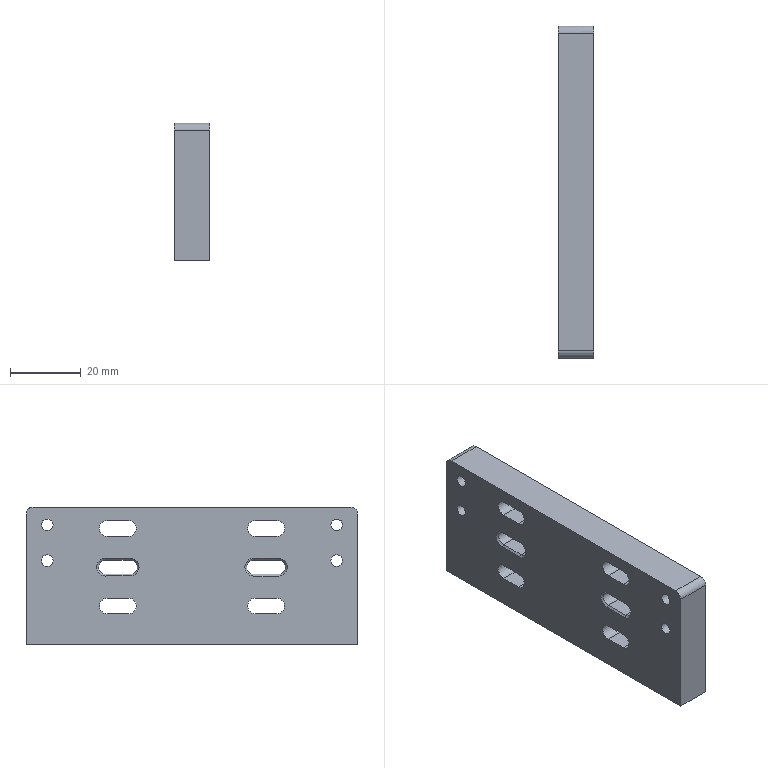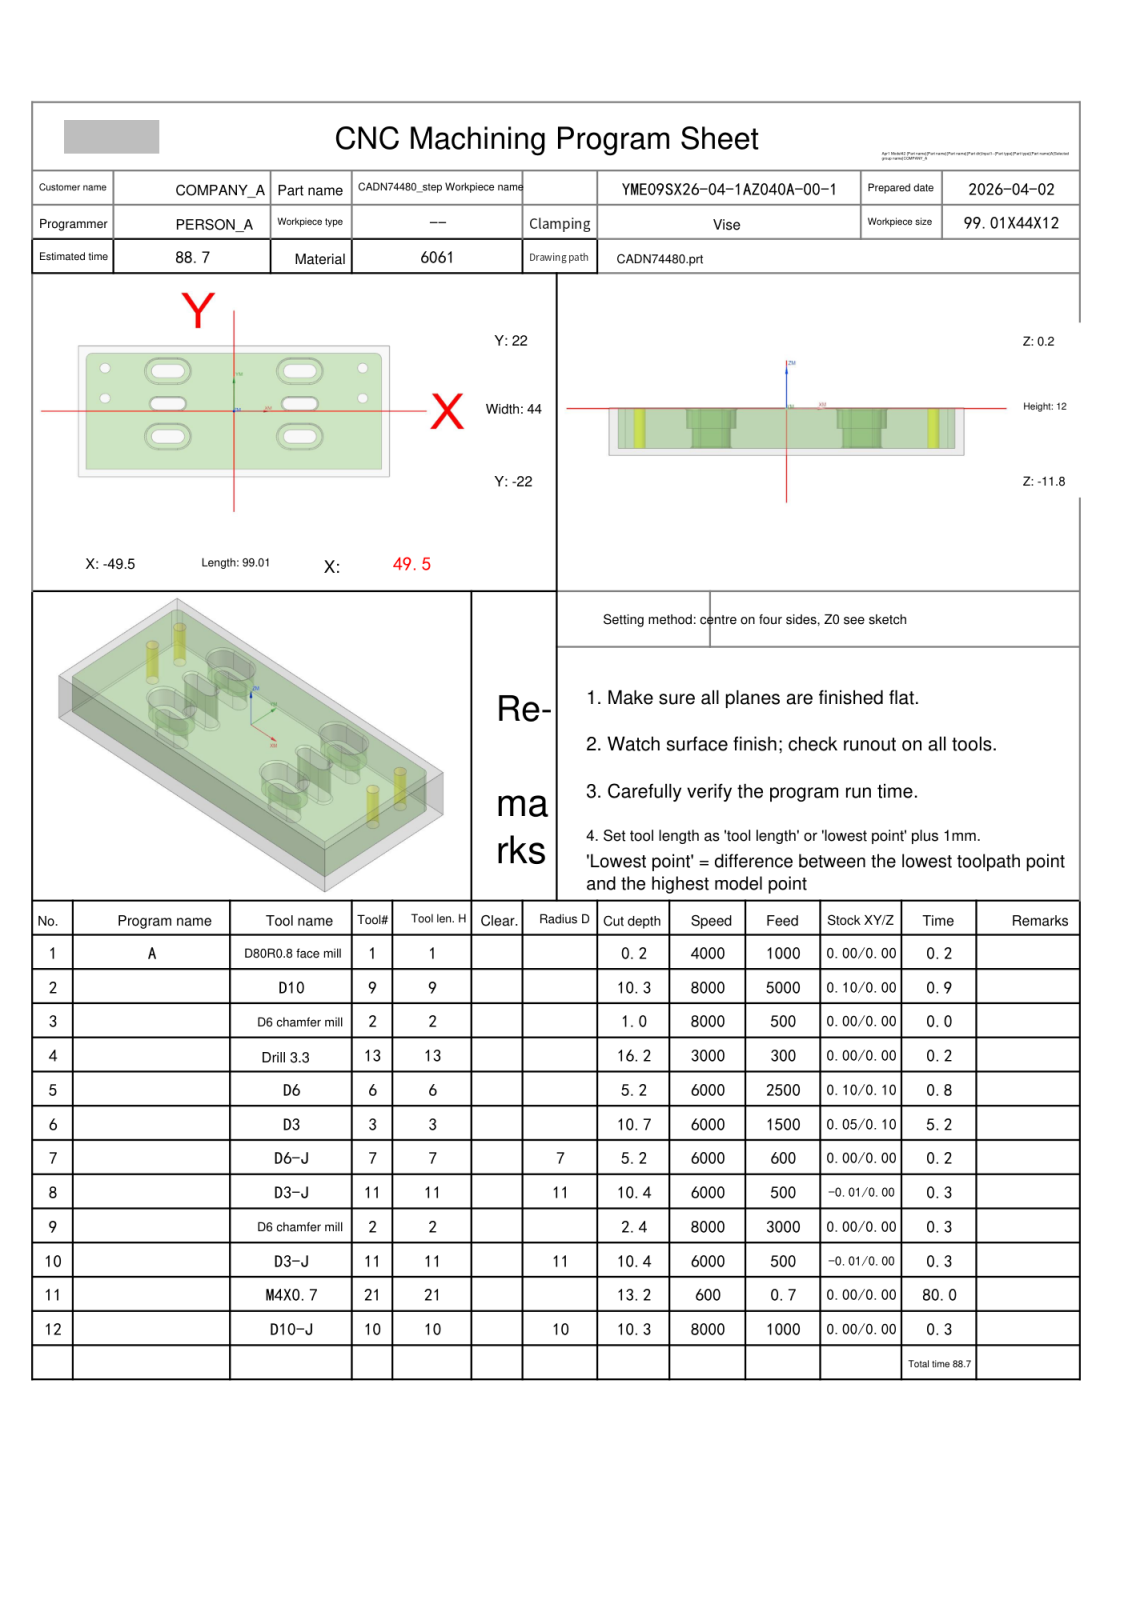NC program | NX | posted by the shop | part box 10.067 x 94 x 39 mm
Lines 3804 to 4590 of 4590:
N7 T07 M06
(D6-J  D=6. R=0. H=07 ce=0.00 di=0.00)
G00 G90 G54 X-21.196 Y-9.25 M03 S6000
G43 H07 Z20.
M08
Z-4.5
G01 Z-5. F600.
G41 D07
Y-9.3
G03 X-20.996 Y-9.5 I.2 J0.0
G01 X-17.996
G03 X-16.996 Y-8.5 I0.0 J1.
X-17.996 Y-7.5 I-1. J0.0
G01 X-23.996
G03 X-24.996 Y-8.5 I0.0 J-1.
X-23.996 Y-9.5 I1. J0.0
G01 X-20.996
X-20.496
G03 X-20.296 Y-9.3 I0.0 J.2
G01 G40 Y-9.25
Z-4.5
G00 Z20.
X-20.796 Y14.25
Z-4.5
G01 Z-5.
G41 D07
Y14.3
G03 X-20.996 Y14.5 I-.2 J0.0
G01 X-23.996
G03 X-24.996 Y13.5 I0.0 J-1.
X-23.996 Y12.5 I1. J0.0
G01 X-17.996
G03 X-16.996 Y13.5 I0.0 J1.
X-17.996 Y14.5 I-1. J0.0
G01 X-20.996
X-21.496
G03 X-21.696 Y14.3 I0.0 J-.2
G01 G40 Y14.25
Z-4.5
G00 Z20.
X21.204
Z-4.5
G01 Z-5.
G41 D07
Y14.3
G03 X21.004 Y14.5 I-.2 J0.0
G01 X18.004
G03 X17.004 Y13.5 I0.0 J-1.
X18.004 Y12.5 I1. J0.0
G01 X24.004
G03 X25.004 Y13.5 I0.0 J1.
X24.004 Y14.5 I-1. J0.0
G01 X21.004
X20.504
G03 X20.304 Y14.3 I0.0 J-.2
G01 G40 Y14.25
Z-4.5
G00 Z20.
X20.804 Y-9.25
Z-4.5
G01 Z-5.
G41 D07
Y-9.3
G03 X21.004 Y-9.5 I.2 J0.0
G01 X24.004
G03 X25.004 Y-8.5 I0.0 J1.
X24.004 Y-7.5 I-1. J0.0
G01 X18.004
G03 X17.004 Y-8.5 I0.0 J-1.
X18.004 Y-9.5 I1. J0.0
G01 X21.004
X21.504
G03 X21.704 Y-9.3 I0.0 J.2
G01 G40 Y-9.25
Z-4.5
G00 Z20.
G91 G28 Z0.0
M05
M09
G91 G28 Z0.0
M01
N8 T11 M06
(D3-J  D=3. R=0. H=11 ce=-0.01 di=0.00)
G00 G90 G54 X-20.796 Y14.01 M03 S6000
G43 H11 Z20.
M08
Z-7.1
G01 Z-7.6 F500.
G41 D07
Y14.06
G03 X-20.996 Y14.26 I-.2 J0.0
G01 X-23.996
G03 X-24.756 Y13.5 I0.0 J-.76
X-23.996 Y12.74 I.76 J0.0
G01 X-17.996
G03 X-17.236 Y13.5 I0.0 J.76
X-17.996 Y14.26 I-.76 J0.0
G01 X-20.996
X-21.496
G03 X-21.696 Y14.06 I0.0 J-.2
G01 G40 Y14.01
Z-7.1
G00 Z-4.
X-20.796
Z-9.7
G01 Z-10.2
G41 D07
Y14.06
G03 X-20.996 Y14.26 I-.2 J0.0
G01 X-23.996
G03 X-24.756 Y13.5 I0.0 J-.76
X-23.996 Y12.74 I.76 J0.0
G01 X-17.996
G03 X-17.236 Y13.5 I0.0 J.76
X-17.996 Y14.26 I-.76 J0.0
G01 X-20.996
X-21.496
G03 X-21.696 Y14.06 I0.0 J-.2
G01 G40 Y14.01
Z-9.7
G00 Z20.
X-21.196 Y-9.01
Z-7.1
G01 Z-7.6
G41 D07
Y-9.06
G03 X-20.996 Y-9.26 I.2 J0.0
G01 X-17.996
G03 X-17.236 Y-8.5 I0.0 J.76
X-17.996 Y-7.74 I-.76 J0.0
G01 X-23.996
G03 X-24.756 Y-8.5 I0.0 J-.76
X-23.996 Y-9.26 I.76 J0.0
G01 X-20.996
X-20.496
G03 X-20.296 Y-9.06 I0.0 J.2
G01 G40 Y-9.01
Z-7.1
G00 Z-4.
X-21.196
Z-9.7
G01 Z-10.2
G41 D07
Y-9.06
G03 X-20.996 Y-9.26 I.2 J0.0
G01 X-17.996
G03 X-17.236 Y-8.5 I0.0 J.76
X-17.996 Y-7.74 I-.76 J0.0
G01 X-23.996
G03 X-24.756 Y-8.5 I0.0 J-.76
X-23.996 Y-9.26 I.76 J0.0
G01 X-20.996
X-20.496
G03 X-20.296 Y-9.06 I0.0 J.2
G01 G40 Y-9.01
Z-9.7
G00 Z20.
X20.804
Z-7.1
G01 Z-7.6
G41 D07
Y-9.06
G03 X21.004 Y-9.26 I.2 J0.0
G01 X24.004
G03 X24.764 Y-8.5 I0.0 J.76
X24.004 Y-7.74 I-.76 J0.0
G01 X18.004
G03 X17.244 Y-8.5 I0.0 J-.76
X18.004 Y-9.26 I.76 J0.0
G01 X21.004
X21.504
G03 X21.704 Y-9.06 I0.0 J.2
G01 G40 Y-9.01
Z-7.1
G00 Z-4.
X20.804
Z-9.7
G01 Z-10.2
G41 D07
Y-9.06
G03 X21.004 Y-9.26 I.2 J0.0
G01 X24.004
G03 X24.764 Y-8.5 I0.0 J.76
X24.004 Y-7.74 I-.76 J0.0
G01 X18.004
G03 X17.244 Y-8.5 I0.0 J-.76
X18.004 Y-9.26 I.76 J0.0
G01 X21.004
X21.504
G03 X21.704 Y-9.06 I0.0 J.2
G01 G40 Y-9.01
Z-9.7
G00 Z20.
X21.204 Y14.01
Z-7.1
G01 Z-7.6
G41 D07
Y14.06
G03 X21.004 Y14.26 I-.2 J0.0
G01 X18.004
G03 X17.244 Y13.5 I0.0 J-.76
X18.004 Y12.74 I.76 J0.0
G01 X24.004
G03 X24.764 Y13.5 I0.0 J.76
X24.004 Y14.26 I-.76 J0.0
G01 X21.004
X20.504
G03 X20.304 Y14.06 I0.0 J-.2
G01 G40 Y14.01
Z-7.1
G00 Z-4.
X21.204
Z-9.7
G01 Z-10.2
G41 D07
Y14.06
G03 X21.004 Y14.26 I-.2 J0.0
G01 X18.004
G03 X17.244 Y13.5 I0.0 J-.76
X18.004 Y12.74 I.76 J0.0
G01 X24.004
G03 X24.764 Y13.5 I0.0 J.76
X24.004 Y14.26 I-.76 J0.0
G01 X21.004
X20.504
G03 X20.304 Y14.06 I0.0 J-.2
G01 G40 Y14.01
Z-9.7
G00 Z20.
G91 G28 Z0.0
M05
M09
G91 G28 Z0.0
M01
N9 T02 M06
(D6 chamfer mill  D=6. R=0. H=02 ce=0.00 di=0.00)
G00 G90 G54 X.253 Y-21.628 M03 S8000
G43 H02 Z20.
M08
Z2.099
G01 Z-1.5 F3000.
G03 X.334 Y-21.328 I-.52 J.3
X.034 Y-20.808 I-.6 J0.0
G01 X.004 Y-20.8
X-46.996
G02 X-48.296 Y-19.5 I0.0 J1.3
G01 Y17.5
X-48.295 Y17.565
X-48.29 Y17.63
X-48.246 Y18.069
X-48.221 Y18.225
X-48.177 Y18.376
X-48.001 Y18.87
X-47.927 Y19.038
X-47.831 Y19.194
X-47.501 Y19.653
X-47.383 Y19.793
X-47.247 Y19.916
X-46.802 Y20.265
X-46.65 Y20.367
X-46.486 Y20.447
X-45.961 Y20.658
X-45.787 Y20.714
X-45.606 Y20.745
X-45.126 Y20.794
X-45.061 Y20.798
X-44.996 Y20.8
X45.004
G02 X45.728 Y20.724 I-.212 J-5.531
G01 X45.88 Y20.681
X46.374 Y20.504
X46.542 Y20.431
X46.698 Y20.334
X47.156 Y20.004
X47.297 Y19.887
X47.42 Y19.751
X47.768 Y19.306
X47.871 Y19.154
X47.951 Y18.989
X48.162 Y18.465
X48.218 Y18.29
X48.249 Y18.11
X48.297 Y17.63
X48.302 Y17.565
X48.304 Y17.5
Y-19.5
G02 X47.004 Y-20.8 I-1.3 J0.0
G01 X.004
X-.026 Y-20.808
G03 X-.326 Y-21.328 I.3 J-.52
X-.246 Y-21.628 I.6 J0.0
G01 Z2.099
G00 Z20.
G00 G90 X41.004 Y4.35 M03 S8000
Z20.
G98 G81 X41.004 Y4.35 Z-2.2 R3. F500.
Y14.5
X-40.996
Y4.35
G80
G00 Z20.
G00 G90 X16.575 Y11.963 M03 S6500
Z20.
Z.3
G01 Z-1.2 F1500.
X16.528 Y11.561
X16.519 Y11.421
G03 X17.579 Y10.229 I1.2 J0.0
X18.019 Y10.2 I.5 J4.248
G01 X23.99
G03 X24.626 Y10.261 I-.094 J4.336
X25.239 Y10.442 I-.626 J3.249
G01 X25.274 Y10.456
G03 X25.616 Y10.623 I-1.271 J3.046
G01 X25.646 Y10.64
X25.734 Y10.692
G03 X26. Y10.874 I-1.737 J2.817
G01 X26.035 Y10.902
X26.134 Y10.983
X26.16 Y11.004
G03 X26.593 Y11.458 I-2.166 J2.505
G01 X26.612 Y11.482
X26.72 Y11.629
X26.736 Y11.653
X26.809 Y11.766
X26.824 Y11.79
X26.887 Y11.899
X26.901 Y11.923
X26.983 Y12.086
X26.998 Y12.118
G03 X27.302 Y13.5 I-2.996 J1.382
X26.123 Y16.027 I-3.299 J0.0
X24.429 Y16.771 I-2.119 J-2.527
G01 X24.211 Y16.792
X23.988 Y16.8
X18.016
G03 X17.385 Y16.74 I.094 J-4.345
X16.668 Y16.516 I.62 J-3.245
G01 X16.625 Y16.497
X16.613 Y16.491
X16.554 Y16.463
X16.508 Y16.44
G03 X16.22 Y16.275 I1.498 J-2.944
G01 X16.189 Y16.255
G03 X15.813 Y15.966 I1.817 J-2.758
G01 X15.787 Y15.942
G03 X15.194 Y15.227 I2.218 J-2.444
G01 X15.178 Y15.202
X15.124 Y15.109
X15.105 Y15.074
X15.084 Y15.036
X15.077 Y15.022
X15.073 Y15.013
X15.05 Y14.969
X14.975 Y14.806
X14.96 Y14.771
G03 X14.705 Y13.5 I3.045 J-1.271
X15.885 Y10.972 I3.299 J0.0
X17.579 Y10.229 I2.121 J2.534
X17.978 Y10.201 I.5 J4.248
G01 X18.006
G03 X19.206 Y11.372 I0.0 J1.2
G01 X19.207 Y11.4
Z.3
G00 Z20.
X16.575 Y-10.037
Z.3
G01 Z-1.2
X16.528 Y-10.439
X16.519 Y-10.579
G03 X17.579 Y-11.771 I1.2 J0.0
X18.019 Y-11.8 I.5 J4.255
G01 X23.99
G03 X24.626 Y-11.739 I-.094 J4.336
G01 X24.744 Y-11.714
X24.782 Y-11.705
G03 X25.274 Y-11.544 I-.78 J3.208
G01 X25.319 Y-11.525
X25.363 Y-11.505
X25.453 Y-11.463
X25.485 Y-11.447
G03 X25.859 Y-11.227 I-1.485 J2.953
G01 X25.897 Y-11.201
X25.934 Y-11.175
G03 X26.176 Y-10.982 I-1.933 J2.679
G01 X26.2 Y-10.96
X26.386 Y-10.78
X26.408 Y-10.758
X26.542 Y-10.606
X26.568 Y-10.575
X26.691 Y-10.412
X26.709 Y-10.387
X26.758 Y-10.315
X26.809 Y-10.234
X26.829 Y-10.202
G03 X27.278 Y-8.895 I-2.827 J1.702
G01 X27.281 Y-8.866
G03 X27.302 Y-8.5 I-3.279 J.365
X25.989 Y-5.867 I-3.299 J0.0
X24.517 Y-5.241 I-2.013 J-2.695
X24.211 Y-5.208 I-.591 J-3.966
G01 X23.988 Y-5.2
X18.016
G03 X17.385 Y-5.26 I.094 J-4.345
X17.107 Y-5.326 I.621 J-3.252
G01 X17.067 Y-5.337
G03 X15.581 Y-6.261 I.937 J-3.163
G01 X15.558 Y-6.286
G03 X15.365 Y-6.521 I2.447 J-2.215
G01 X15.327 Y-6.573
X15.296 Y-6.616
X15.273 Y-6.65
G03 X15.1 Y-6.935 I2.764 J-1.871
G01 X15.086 Y-6.96
X14.967 Y-7.211
X14.953 Y-7.246
G03 X14.705 Y-8.5 I3.052 J-1.254
X15.885 Y-11.028 I3.299 J0.0
X17.579 Y-11.771 I2.121 J2.534
X17.978 Y-11.799 I.5 J4.255
G01 X18.007
G03 X19.206 Y-10.628 I0.0 J1.2
G01 X19.207 Y-10.6
Z.3
G00 Z20.
X-25.425 Y-10.037
Z.3
G01 Z-1.2
X-25.473 Y-10.439
X-25.481 Y-10.579
G03 X-24.421 Y-11.771 I1.2 J0.0
X-23.981 Y-11.8 I.501 J4.262
G01 X-18.01
G03 X-17.374 Y-11.739 I-.094 J4.336
X-16.738 Y-11.549 I-.623 J3.242
G01 X-16.704 Y-11.534
G03 X-16.247 Y-11.296 I-1.294 J3.036
G01 X-16.217 Y-11.277
X-16.009 Y-11.133
X-15.983 Y-11.112
X-15.832 Y-10.989
X-15.8 Y-10.96
X-15.713 Y-10.88
G03 X-15.471 Y-10.621 I-2.288 J2.384
G01 X-15.451 Y-10.598
X-15.413 Y-10.551
X-15.394 Y-10.526
X-15.264 Y-10.347
X-15.248 Y-10.322
X-15.232 Y-10.299
G03 X-14.698 Y-8.499 I-2.769 J1.8
G01 Y-8.473
X-14.699 Y-8.444
G03 X-16.011 Y-5.867 I-3.299 J-.056
X-17.611 Y-5.224 I-2.015 J-2.703
G01 X-17.789 Y-5.208
X-17.829 Y-5.205
X-17.91 Y-5.203
X-23.984 Y-5.2
G03 X-24.615 Y-5.26 I.094 J-4.344
X-25.78 Y-5.725 I.619 J-3.242
G01 X-25.811 Y-5.745
X-25.897 Y-5.804
G03 X-26.326 Y-6.165 I1.902 J-2.698
G01 X-26.35 Y-6.189
G03 X-26.886 Y-6.909 I2.355 J-2.312
G01 X-26.9 Y-6.935
X-26.946 Y-7.023
X-26.959 Y-7.049
X-27.018 Y-7.176
X-27.029 Y-7.202
G03 X-27.295 Y-8.5 I3.033 J-1.297
X-26.115 Y-11.028 I3.299 J0.0
X-24.421 Y-11.771 I2.121 J2.534
X-24.022 Y-11.799 I.501 J4.262
G01 X-23.993
G03 X-22.794 Y-10.628 I0.0 J1.2
G01 X-22.793 Y-10.6
Z.3
G00 Z20.
X-16.646 Y15.106
Z.3
G01 Z-1.2
X-16.631 Y15.551
X-16.63 Y15.593
G03 X-17.789 Y16.792 I-1.2 J0.0
G01 X-18.012 Y16.8
X-23.984
G03 X-24.615 Y16.74 I.094 J-4.344
X-25.399 Y16.486 I.619 J-3.244
G01 X-25.434 Y16.469
X-25.548 Y16.411
X-25.594 Y16.386
X-25.705 Y16.322
X-25.737 Y16.302
G03 X-26.179 Y15.974 I1.742 J-2.803
G01 X-26.205 Y15.95
G03 X-26.442 Y15.714 I2.212 J-2.454
G01 X-26.464 Y15.689
G03 X-26.654 Y15.453 I2.473 J-2.193
G01 X-26.673 Y15.427
X-26.692 Y15.401
X-26.739 Y15.332
X-26.774 Y15.279
X-26.796 Y15.245
X-26.812 Y15.219
G03 X-27.025 Y14.806 I2.826 J-1.724
G01 X-27.036 Y14.78
G03 X-27.258 Y13.989 I3.043 J-1.281
G01 X-27.263 Y13.956
X-27.268 Y13.924
G03 X-27.295 Y13.501 I3.272 J-.423
X-25.982 Y10.866 I3.3 J0.0
X-24.364 Y10.222 I2.011 J2.699
X-23.981 Y10.2 I.452 J4.583
G01 X-18.01
G03 X-17.374 Y10.261 I-.094 J4.336
X-16.58 Y10.521 I-.623 J3.241
G01 X-16.547 Y10.537
X-16.504 Y10.559
X-16.266 Y10.692
X-16.237 Y10.71
X-16.16 Y10.76
X-16.112 Y10.793
X-16.076 Y10.819
G03 X-15.599 Y11.235 I-1.923 J2.684
G01 X-15.578 Y11.258
G03 X-15.264 Y11.653 I-2.422 J2.245
G01 X-15.248 Y11.678
X-15.186 Y11.774
X-15.166 Y11.807
X-15.147 Y11.839
G03 X-14.7 Y13.499 I-2.86 J1.66
X-15.524 Y15.683 I-3.307 J0.0
X-16.909 Y16.614 I-2.474 J-2.185
X-17.789 Y16.792 I-1.125 J-3.29
G01 X-18.012 Y16.8
X-18.188
G03 X-19.388 Y15.6 I0.0 J-1.2
G01 Z.3
G00 Z20.
G00 G90 X-16.678 Y1.491 M03 S7000
Z20.
Z2.5
G01 X-16.554 Y1.604 Z2.439 F1500.
X-16.44 Y1.743 Z2.374
X-16.345 Y1.896 Z2.308
X-16.273 Y2.061 Z2.243
X-16.224 Y2.234 Z2.177
X-16.199 Y2.412 Z2.112
X-16.2 Y2.592 Z2.046
X-16.225 Y2.77 Z1.981
X-16.274 Y2.943 Z1.915
X-16.347 Y3.107 Z1.85
X-16.442 Y3.26 Z1.784
X-16.557 Y3.399 Z1.719
X-16.69 Y3.52 Z1.653
X-16.839 Y3.621 Z1.588
X-17. Y3.701 Z1.523
X-17.17 Y3.758 Z1.457
X-17.345 Y3.791 Z1.392
X-17.526 Y3.8 Z1.326
X-24.467 Z-1.2
X-24.496
G03 X-25.797 Y2.5 I0.0 J-1.3
X-25.646 Y1.893 I1.3 J0.0
X-24.496 Y1.2 I1.15 J.608
G01 X-24.467
X-17.526
X-17.497
G03 X-16.196 Y2.5 I0.0 J1.3
X-16.347 Y3.107 I-1.3 J0.0
X-17.497 Y3.8 I-1.15 J-.608
G01 X-17.526
X-24.467
X-24.65 Y3.791
X-24.827 Y3.758
X-24.957 Y3.714
Z1.3
G00 Z20.
X25.322 Y1.491
Z2.5
G01 X25.446 Y1.604 Z2.439
X25.56 Y1.743 Z2.374
X25.655 Y1.896 Z2.308
X25.727 Y2.061 Z2.243
X25.776 Y2.234 Z2.177
X25.801 Y2.412 Z2.112
X25.8 Y2.592 Z2.046
X25.775 Y2.77 Z1.981
X25.726 Y2.943 Z1.915
X25.653 Y3.107 Z1.85
X25.558 Y3.26 Z1.784
X25.443 Y3.399 Z1.719
X25.31 Y3.52 Z1.653
X25.161 Y3.621 Z1.588
X25. Y3.701 Z1.523
X24.83 Y3.758 Z1.457
X24.655 Y3.791 Z1.392
X24.474 Y3.8 Z1.326
X17.533 Z-1.2
X17.504
G03 X16.203 Y2.5 I0.0 J-1.3
X16.354 Y1.893 I1.3 J0.0
X17.504 Y1.2 I1.15 J.608
G01 X17.533
X24.474
X24.503
G03 X25.804 Y2.5 I0.0 J1.3
X25.653 Y3.107 I-1.3 J0.0
X24.503 Y3.8 I-1.15 J-.608
G01 X24.474
X17.533
X17.35 Y3.791
X17.173 Y3.758
X17.043 Y3.714
Z1.3
G00 Z20.
G91 G28 Z0.0
M05
M09
G91 G28 Z0.0
M01
N10 T11 M06
(D3-J  D=3. R=0. H=11 ce=-0.01 di=0.00)
G00 G90 G54 X21.204 Y2.76 M03 S6000
G43 H11 Z20.
M08
Z-2.9
G01 Z-3.4 F500.
G41 D07
Y2.81
G03 X21.004 Y3.01 I-.2 J0.0
G01 X17.504
G03 X16.994 Y2.5 I0.0 J-.51
X17.504 Y1.99 I.51 J0.0
G01 X24.504
G03 X25.014 Y2.5 I0.0 J.51
X24.504 Y3.01 I-.51 J0.0
G01 X21.004
X20.504
G03 X20.304 Y2.81 I0.0 J-.2
G01 G40 Y2.76
Z-2.9
G00 Z1.
X21.204
Z-6.3
G01 Z-6.8
G41 D07
Y2.81
G03 X21.004 Y3.01 I-.2 J0.0
G01 X17.504
G03 X16.994 Y2.5 I0.0 J-.51
X17.504 Y1.99 I.51 J0.0
G01 X24.504
G03 X25.014 Y2.5 I0.0 J.51
X24.504 Y3.01 I-.51 J0.0
G01 X21.004
X20.504
G03 X20.304 Y2.81 I0.0 J-.2
G01 G40 Y2.76
Z-6.3
G00 Z-2.4
X21.204
Z-9.7
G01 Z-10.2
G41 D07
Y2.81
G03 X21.004 Y3.01 I-.2 J0.0
G01 X17.504
G03 X16.994 Y2.5 I0.0 J-.51
X17.504 Y1.99 I.51 J0.0
G01 X24.504
G03 X25.014 Y2.5 I0.0 J.51
X24.504 Y3.01 I-.51 J0.0
G01 X21.004
X20.504
G03 X20.304 Y2.81 I0.0 J-.2
G01 G40 Y2.76
Z-9.7
G00 Z20.
X-20.796
Z-2.9
G01 Z-3.4
G41 D07
Y2.81
G03 X-20.996 Y3.01 I-.2 J0.0
G01 X-24.496
G03 X-25.006 Y2.5 I0.0 J-.51
X-24.496 Y1.99 I.51 J0.0
G01 X-17.496
G03 X-16.986 Y2.5 I0.0 J.51
X-17.496 Y3.01 I-.51 J0.0
G01 X-20.996
X-21.496
G03 X-21.696 Y2.81 I0.0 J-.2
G01 G40 Y2.76
Z-2.9
G00 Z1.
X-20.796
Z-6.3
G01 Z-6.8
G41 D07
Y2.81
G03 X-20.996 Y3.01 I-.2 J0.0
G01 X-24.496
G03 X-25.006 Y2.5 I0.0 J-.51
X-24.496 Y1.99 I.51 J0.0
G01 X-17.496
G03 X-16.986 Y2.5 I0.0 J.51
X-17.496 Y3.01 I-.51 J0.0
G01 X-20.996
X-21.496
G03 X-21.696 Y2.81 I0.0 J-.2
G01 G40 Y2.76
Z-6.3
G00 Z-2.4
X-20.796
Z-9.7
G01 Z-10.2
G41 D07
Y2.81
G03 X-20.996 Y3.01 I-.2 J0.0
G01 X-24.496
G03 X-25.006 Y2.5 I0.0 J-.51
X-24.496 Y1.99 I.51 J0.0
G01 X-17.496
G03 X-16.986 Y2.5 I0.0 J.51
X-17.496 Y3.01 I-.51 J0.0
G01 X-20.996
X-21.496
G03 X-21.696 Y2.81 I0.0 J-.2
G01 G40 Y2.76
Z-9.7
G00 Z20.
G91 G28 Z0.0
M05
M09
G91 G28 Z0.0
M01
N11 T21 M06
(M4X0.7 D=3.3 DR_a=180 H=21)
G00 G90 G54 X41.004 Y4.35 M03 S600
G43 H21 Z20.
M08
G95
G98 G84 X41.004 Y4.35 Z-13. R1. F.7 Q4.
Y14.5
X-40.996
Y4.35
G80
G94
G00 Z20.
G91 G28 Z0.0
M05
M09
G91 G28 Z0.0
M01
N12 T10 M06
(D10-J  D=10. R=0. H=10 ce=0.00 di=0.00)
G00 G90 G54 X48.017 Y-25.616 M03 S8000
G43 H10 Z20.
M08
Z-9.6
G01 Z-10.1 F1000.
G41 D10
X48. Y-25.417
G03 X47.004 Y-24.5 I-.997 J-.083
G01 X-47.004
G02 X-52.004 Y-19.5 I0.0 J5.
G01 Y17.5
G02 X-45.004 Y24.5 I7. J0.0
G01 X45.004
G02 X52.004 Y17.5 I0.0 J-7.
G01 Y-19.5
G02 X47.004 Y-24.5 I-5. J0.0
G01 X46.504
G03 X45.504 Y-25.5 I0.0 J-1.
G01 G40 Y-25.7
Z-9.6
G00 Z20.
M05
M09
G91 G28 Z0.0
G91 G28 Y0.0
M30
%